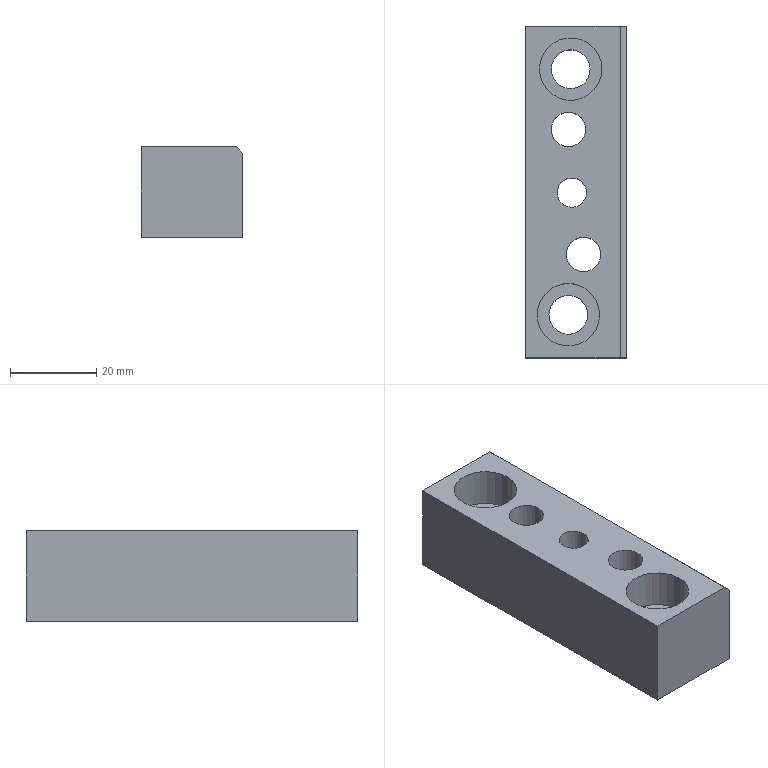Part | NX | features 23 2 | 1 solid | 16 faces | box 23.541 x 77 x 21 mm | volume 30606 mm3 | plane 9 | cylinder 7 | commonest cylinder face diameters 8.001 x2 9 x2 14.5 x2 6.8 x1
STEP:
#1=CARTESIAN_POINT('',(1071.25,287.,-2.5));
#2=VERTEX_POINT('',#1);
#3=CARTESIAN_POINT('',(1064.,287.,-2.5));
#4=DIRECTION('',(0.,0.,1.));
#5=DIRECTION('',(1.,0.,0.));
#6=AXIS2_PLACEMENT_3D('',#3,#4,#5);
#7=CIRCLE('',#6,7.25);
#8=EDGE_CURVE('',#2,#2,#7,.T.);
#9=ORIENTED_EDGE('',*,*,#8,.F.);
#10=EDGE_LOOP('',(#9));
#11=FACE_BOUND('',#10,.T.);
#12=CARTESIAN_POINT('',(1071.542,301.,-2.5));
#13=VERTEX_POINT('',#12);
#14=CARTESIAN_POINT('',(1067.541,301.,-2.5));
#15=DIRECTION('',(0.,0.,-1.));
#16=DIRECTION('',(1.,0.,0.));
#17=AXIS2_PLACEMENT_3D('',#14,#15,#16);
#18=CIRCLE('',#17,4.);
#19=EDGE_CURVE('',#13,#13,#18,.T.);
#20=ORIENTED_EDGE('',*,*,#19,.T.);
#21=EDGE_LOOP('',(#20));
#22=FACE_BOUND('',#21,.T.);
#23=CARTESIAN_POINT('',(1076.041,277.,-2.5));
#24=VERTEX_POINT('',#23);
#25=CARTESIAN_POINT('',(1076.041,354.,-2.5));
#26=VERTEX_POINT('',#25);
#27=CARTESIAN_POINT('',(1076.041,-425.,-2.5));
#28=DIRECTION('',(0.,1.,0.));
#29=VECTOR('',#28,1000.);
#30=LINE('',#27,#29);
#31=EDGE_CURVE('',#24,#26,#30,.T.);
#32=ORIENTED_EDGE('',*,*,#31,.T.);
#33=CARTESIAN_POINT('',(1054.,354.,-2.5));
#34=VERTEX_POINT('',#33);
#35=CARTESIAN_POINT('',(1166.5,354.,-2.5));
#36=DIRECTION('',(1.,0.,0.));
#37=VECTOR('',#36,1000.);
#38=LINE('',#35,#37);
#39=EDGE_CURVE('',#34,#26,#38,.T.);
#40=ORIENTED_EDGE('',*,*,#39,.F.);
#41=CARTESIAN_POINT('',(1054.,277.,-2.5));
#42=VERTEX_POINT('',#41);
#43=CARTESIAN_POINT('',(1054.,328.5,-2.5));
#44=DIRECTION('',(0.,-1.,0.));
#45=VECTOR('',#44,1000.);
#46=LINE('',#43,#45);
#47=EDGE_CURVE('',#34,#42,#46,.T.);
#48=ORIENTED_EDGE('',*,*,#47,.T.);
#49=CARTESIAN_POINT('',(1166.5,277.,-2.5));
#50=DIRECTION('',(1.,0.,0.));
#51=VECTOR('',#50,1000.);
#52=LINE('',#49,#51);
#53=EDGE_CURVE('',#42,#24,#52,.T.);
#54=ORIENTED_EDGE('',*,*,#53,.T.);
#55=EDGE_LOOP('',(#32,#40,#48,#54));
#56=FACE_BOUND('',#55,.T.);
#57=CARTESIAN_POINT('',(1071.791,344.,-2.5));
#58=VERTEX_POINT('',#57);
#59=CARTESIAN_POINT('',(1064.541,344.,-2.5));
#60=DIRECTION('',(0.,0.,1.));
#61=DIRECTION('',(1.,0.,0.));
#62=AXIS2_PLACEMENT_3D('',#59,#60,#61);
#63=CIRCLE('',#62,7.25);
#64=EDGE_CURVE('',#58,#58,#63,.T.);
#65=ORIENTED_EDGE('',*,*,#64,.F.);
#66=EDGE_LOOP('',(#65));
#67=FACE_BOUND('',#66,.T.);
#68=CARTESIAN_POINT('',(1068.001,330.,-2.5));
#69=VERTEX_POINT('',#68);
#70=CARTESIAN_POINT('',(1064.,330.,-2.5));
#71=DIRECTION('',(0.,0.,-1.));
#72=DIRECTION('',(1.,0.,0.));
#73=AXIS2_PLACEMENT_3D('',#70,#71,#72);
#74=CIRCLE('',#73,4.);
#75=EDGE_CURVE('',#69,#69,#74,.T.);
#76=ORIENTED_EDGE('',*,*,#75,.T.);
#77=EDGE_LOOP('',(#76));
#78=FACE_BOUND('',#77,.T.);
#79=CARTESIAN_POINT('',(1068.223,315.331,-2.5));
#80=VERTEX_POINT('',#79);
#81=CARTESIAN_POINT('',(1064.823,315.331,-2.5));
#82=DIRECTION('',(0.,0.,1.));
#83=DIRECTION('',(1.,0.,0.));
#84=AXIS2_PLACEMENT_3D('',#81,#82,#83);
#85=CIRCLE('',#84,3.4);
#86=EDGE_CURVE('',#80,#80,#85,.T.);
#87=ORIENTED_EDGE('',*,*,#86,.F.);
#88=EDGE_LOOP('',(#87));
#89=FACE_BOUND('',#88,.T.);
#90=CARTESIAN_POINT('',(1166.5,279.5,-2.5));
#91=DIRECTION('',(0.,0.,1.));
#92=DIRECTION('',(-1.,0.,0.));
#93=AXIS2_PLACEMENT_3D('',#90,#91,#92);
#94=PLANE('',#93);
#95=ADVANCED_FACE('',(#11,#22,#56,#67,#78,#89),#94,.T.);
#96=CARTESIAN_POINT('',(1054.,354.,-23.5));
#97=VERTEX_POINT('',#96);
#98=CARTESIAN_POINT('',(1054.,354.,-33.5));
#99=DIRECTION('',(0.,0.,-1.));
#100=VECTOR('',#99,1000.);
#101=LINE('',#98,#100);
#102=EDGE_CURVE('',#34,#97,#101,.T.);
#103=ORIENTED_EDGE('',*,*,#102,.F.);
#104=ORIENTED_EDGE('',*,*,#39,.T.);
#105=CARTESIAN_POINT('',(1077.541,354.,-4.));
#106=VERTEX_POINT('',#105);
#107=CARTESIAN_POINT('',(1077.041,354.,-3.5));
#108=DIRECTION('',(0.7071,0.,-0.7071));
#109=VECTOR('',#108,1000.);
#110=LINE('',#107,#109);
#111=EDGE_CURVE('',#26,#106,#110,.T.);
#112=ORIENTED_EDGE('',*,*,#111,.T.);
#113=CARTESIAN_POINT('',(1077.541,354.,-23.5));
#114=VERTEX_POINT('',#113);
#115=CARTESIAN_POINT('',(1077.541,354.,-43.));
#116=DIRECTION('',(0.,0.,1.));
#117=VECTOR('',#116,1000.);
#118=LINE('',#115,#117);
#119=EDGE_CURVE('',#114,#106,#118,.T.);
#120=ORIENTED_EDGE('',*,*,#119,.F.);
#121=CARTESIAN_POINT('',(1136.,354.,-23.5));
#122=DIRECTION('',(-1.,0.,0.));
#123=VECTOR('',#122,1000.);
#124=LINE('',#121,#123);
#125=EDGE_CURVE('',#114,#97,#124,.T.);
#126=ORIENTED_EDGE('',*,*,#125,.T.);
#127=EDGE_LOOP('',(#103,#104,#112,#120,#126));
#128=FACE_BOUND('',#127,.T.);
#129=CARTESIAN_POINT('',(1033.,354.,0.));
#130=DIRECTION('',(0.,1.,0.));
#131=DIRECTION('',(0.,0.,-1.));
#132=AXIS2_PLACEMENT_3D('',#129,#130,#131);
#133=PLANE('',#132);
#134=ADVANCED_FACE('',(#128),#133,.T.);
#135=CARTESIAN_POINT('',(1054.,277.,-23.5));
#136=VERTEX_POINT('',#135);
#137=CARTESIAN_POINT('',(1054.,277.,-33.5));
#138=DIRECTION('',(0.,0.,-1.));
#139=VECTOR('',#138,1000.);
#140=LINE('',#137,#139);
#141=EDGE_CURVE('',#42,#136,#140,.T.);
#142=ORIENTED_EDGE('',*,*,#141,.T.);
#143=CARTESIAN_POINT('',(1077.541,277.,-23.5));
#144=VERTEX_POINT('',#143);
#145=CARTESIAN_POINT('',(1136.,277.,-23.5));
#146=DIRECTION('',(-1.,0.,0.));
#147=VECTOR('',#146,1000.);
#148=LINE('',#145,#147);
#149=EDGE_CURVE('',#144,#136,#148,.T.);
#150=ORIENTED_EDGE('',*,*,#149,.F.);
#151=CARTESIAN_POINT('',(1077.541,277.,-4.));
#152=VERTEX_POINT('',#151);
#153=CARTESIAN_POINT('',(1077.541,277.,-43.));
#154=DIRECTION('',(0.,0.,-1.));
#155=VECTOR('',#154,1000.);
#156=LINE('',#153,#155);
#157=EDGE_CURVE('',#152,#144,#156,.T.);
#158=ORIENTED_EDGE('',*,*,#157,.F.);
#159=CARTESIAN_POINT('',(1077.041,277.,-3.5));
#160=DIRECTION('',(-0.7071,0.,0.7071));
#161=VECTOR('',#160,1000.);
#162=LINE('',#159,#161);
#163=EDGE_CURVE('',#152,#24,#162,.T.);
#164=ORIENTED_EDGE('',*,*,#163,.T.);
#165=ORIENTED_EDGE('',*,*,#53,.F.);
#166=EDGE_LOOP('',(#142,#150,#158,#164,#165));
#167=FACE_BOUND('',#166,.T.);
#168=CARTESIAN_POINT('',(1027.,277.,0.));
#169=DIRECTION('',(0.,1.,0.));
#170=DIRECTION('',(0.,0.,-1.));
#171=AXIS2_PLACEMENT_3D('',#168,#169,#170);
#172=PLANE('',#171);
#173=ADVANCED_FACE('',(#167),#172,.F.);
#174=CARTESIAN_POINT('',(1077.541,328.5,-23.5));
#175=DIRECTION('',(0.,-1.,0.));
#176=VECTOR('',#175,1000.);
#177=LINE('',#174,#176);
#178=EDGE_CURVE('',#114,#144,#177,.T.);
#179=ORIENTED_EDGE('',*,*,#178,.F.);
#180=ORIENTED_EDGE('',*,*,#119,.T.);
#181=CARTESIAN_POINT('',(1077.541,-425.,-4.));
#182=DIRECTION('',(0.,-1.,0.));
#183=VECTOR('',#182,1000.);
#184=LINE('',#181,#183);
#185=EDGE_CURVE('',#106,#152,#184,.T.);
#186=ORIENTED_EDGE('',*,*,#185,.T.);
#187=ORIENTED_EDGE('',*,*,#157,.T.);
#188=EDGE_LOOP('',(#179,#180,#186,#187));
#189=FACE_BOUND('',#188,.T.);
#190=CARTESIAN_POINT('',(1077.541,275.983,-43.));
#191=DIRECTION('',(1.,0.,0.));
#192=DIRECTION('',(0.,0.,1.));
#193=AXIS2_PLACEMENT_3D('',#190,#191,#192);
#194=PLANE('',#193);
#195=ADVANCED_FACE('',(#189),#194,.T.);
#196=ORIENTED_EDGE('',*,*,#185,.F.);
#197=ORIENTED_EDGE('',*,*,#111,.F.);
#198=ORIENTED_EDGE('',*,*,#31,.F.);
#199=ORIENTED_EDGE('',*,*,#163,.F.);
#200=EDGE_LOOP('',(#196,#197,#198,#199));
#201=FACE_BOUND('',#200,.T.);
#202=CARTESIAN_POINT('',(1077.041,-425.,-3.5));
#203=DIRECTION('',(0.7071,0.,0.7071));
#204=DIRECTION('',(0.,-1.,0.));
#205=AXIS2_PLACEMENT_3D('',#202,#203,#204);
#206=PLANE('',#205);
#207=ADVANCED_FACE('',(#201),#206,.T.);
#208=ORIENTED_EDGE('',*,*,#47,.F.);
#209=ORIENTED_EDGE('',*,*,#102,.T.);
#210=CARTESIAN_POINT('',(1054.,328.5,-23.5));
#211=DIRECTION('',(0.,1.,0.));
#212=VECTOR('',#211,1000.);
#213=LINE('',#210,#212);
#214=EDGE_CURVE('',#136,#97,#213,.T.);
#215=ORIENTED_EDGE('',*,*,#214,.F.);
#216=ORIENTED_EDGE('',*,*,#141,.F.);
#217=EDGE_LOOP('',(#208,#209,#215,#216));
#218=FACE_BOUND('',#217,.T.);
#219=CARTESIAN_POINT('',(1054.,328.5,-33.5));
#220=DIRECTION('',(-1.,0.,0.));
#221=DIRECTION('',(0.,0.,-1.));
#222=AXIS2_PLACEMENT_3D('',#219,#220,#221);
#223=PLANE('',#222);
#224=ADVANCED_FACE('',(#218),#223,.T.);
#225=CARTESIAN_POINT('',(1061.423,315.331,-23.5));
#226=VERTEX_POINT('',#225);
#227=CARTESIAN_POINT('',(1064.823,315.331,-23.5));
#228=DIRECTION('',(0.,0.,1.));
#229=DIRECTION('',(-1.,0.,0.));
#230=AXIS2_PLACEMENT_3D('',#227,#228,#229);
#231=CIRCLE('',#230,3.4);
#232=EDGE_CURVE('',#226,#226,#231,.T.);
#233=ORIENTED_EDGE('',*,*,#232,.T.);
#234=EDGE_LOOP('',(#233));
#235=FACE_BOUND('',#234,.T.);
#236=CARTESIAN_POINT('',(1059.999,330.,-23.5));
#237=VERTEX_POINT('',#236);
#238=CARTESIAN_POINT('',(1064.,330.,-23.5));
#239=DIRECTION('',(0.,0.,1.));
#240=DIRECTION('',(-1.,0.,0.));
#241=AXIS2_PLACEMENT_3D('',#238,#239,#240);
#242=CIRCLE('',#241,4.);
#243=EDGE_CURVE('',#237,#237,#242,.T.);
#244=ORIENTED_EDGE('',*,*,#243,.T.);
#245=EDGE_LOOP('',(#244));
#246=FACE_BOUND('',#245,.T.);
#247=CARTESIAN_POINT('',(1059.5,287.,-23.5));
#248=VERTEX_POINT('',#247);
#249=CARTESIAN_POINT('',(1064.,287.,-23.5));
#250=DIRECTION('',(0.,0.,1.));
#251=DIRECTION('',(-1.,0.,0.));
#252=AXIS2_PLACEMENT_3D('',#249,#250,#251);
#253=CIRCLE('',#252,4.5);
#254=EDGE_CURVE('',#248,#248,#253,.T.);
#255=ORIENTED_EDGE('',*,*,#254,.T.);
#256=EDGE_LOOP('',(#255));
#257=FACE_BOUND('',#256,.T.);
#258=CARTESIAN_POINT('',(1063.541,301.,-23.5));
#259=VERTEX_POINT('',#258);
#260=CARTESIAN_POINT('',(1067.541,301.,-23.5));
#261=DIRECTION('',(0.,0.,1.));
#262=DIRECTION('',(-1.,0.,0.));
#263=AXIS2_PLACEMENT_3D('',#260,#261,#262);
#264=CIRCLE('',#263,4.);
#265=EDGE_CURVE('',#259,#259,#264,.T.);
#266=ORIENTED_EDGE('',*,*,#265,.T.);
#267=EDGE_LOOP('',(#266));
#268=FACE_BOUND('',#267,.T.);
#269=CARTESIAN_POINT('',(1060.041,344.,-23.5));
#270=VERTEX_POINT('',#269);
#271=CARTESIAN_POINT('',(1064.541,344.,-23.5));
#272=DIRECTION('',(0.,0.,1.));
#273=DIRECTION('',(-1.,0.,0.));
#274=AXIS2_PLACEMENT_3D('',#271,#272,#273);
#275=CIRCLE('',#274,4.5);
#276=EDGE_CURVE('',#270,#270,#275,.T.);
#277=ORIENTED_EDGE('',*,*,#276,.T.);
#278=EDGE_LOOP('',(#277));
#279=FACE_BOUND('',#278,.T.);
#280=ORIENTED_EDGE('',*,*,#214,.T.);
#281=ORIENTED_EDGE('',*,*,#125,.F.);
#282=ORIENTED_EDGE('',*,*,#178,.T.);
#283=ORIENTED_EDGE('',*,*,#149,.T.);
#284=EDGE_LOOP('',(#280,#281,#282,#283));
#285=FACE_BOUND('',#284,.T.);
#286=CARTESIAN_POINT('',(1136.,328.5,-23.5));
#287=DIRECTION('',(0.,0.,-1.));
#288=DIRECTION('',(1.,0.,0.));
#289=AXIS2_PLACEMENT_3D('',#286,#287,#288);
#290=PLANE('',#289);
#291=ADVANCED_FACE('',(#235,#246,#257,#268,#279,#285),#290,.T.);
#292=ORIENTED_EDGE('',*,*,#276,.F.);
#293=EDGE_LOOP('',(#292));
#294=FACE_BOUND('',#293,.T.);
#295=CARTESIAN_POINT('',(1060.041,344.,-11.5));
#296=VERTEX_POINT('',#295);
#297=CARTESIAN_POINT('',(1064.541,344.,-11.5));
#298=DIRECTION('',(0.,0.,1.));
#299=DIRECTION('',(-1.,0.,0.));
#300=AXIS2_PLACEMENT_3D('',#297,#298,#299);
#301=CIRCLE('',#300,4.5);
#302=EDGE_CURVE('',#296,#296,#301,.T.);
#303=ORIENTED_EDGE('',*,*,#302,.T.);
#304=EDGE_LOOP('',(#303));
#305=FACE_BOUND('',#304,.T.);
#306=CARTESIAN_POINT('',(1064.541,344.,-0.5));
#307=DIRECTION('',(0.,0.,-1.));
#308=DIRECTION('',(-1.,0.,0.));
#309=AXIS2_PLACEMENT_3D('',#306,#307,#308);
#310=CYLINDRICAL_SURFACE('',#309,4.5);
#311=ADVANCED_FACE('',(#294,#305),#310,.F.);
#312=ORIENTED_EDGE('',*,*,#302,.F.);
#313=EDGE_LOOP('',(#312));
#314=FACE_BOUND('',#313,.T.);
#315=CARTESIAN_POINT('',(1057.291,344.,-11.5));
#316=VERTEX_POINT('',#315);
#317=CARTESIAN_POINT('',(1064.541,344.,-11.5));
#318=DIRECTION('',(0.,0.,1.));
#319=DIRECTION('',(-1.,0.,0.));
#320=AXIS2_PLACEMENT_3D('',#317,#318,#319);
#321=CIRCLE('',#320,7.25);
#322=EDGE_CURVE('',#316,#316,#321,.T.);
#323=ORIENTED_EDGE('',*,*,#322,.T.);
#324=EDGE_LOOP('',(#323));
#325=FACE_BOUND('',#324,.T.);
#326=CARTESIAN_POINT('',(1064.541,344.,-11.5));
#327=DIRECTION('',(0.,0.,-1.));
#328=DIRECTION('',(1.,0.,0.));
#329=AXIS2_PLACEMENT_3D('',#326,#327,#328);
#330=PLANE('',#329);
#331=ADVANCED_FACE('',(#314,#325),#330,.F.);
#332=ORIENTED_EDGE('',*,*,#322,.F.);
#333=EDGE_LOOP('',(#332));
#334=FACE_BOUND('',#333,.T.);
#335=ORIENTED_EDGE('',*,*,#64,.T.);
#336=EDGE_LOOP('',(#335));
#337=FACE_BOUND('',#336,.T.);
#338=CARTESIAN_POINT('',(1064.541,344.,-2.5));
#339=DIRECTION('',(0.,0.,-1.));
#340=DIRECTION('',(-1.,0.,0.));
#341=AXIS2_PLACEMENT_3D('',#338,#339,#340);
#342=CYLINDRICAL_SURFACE('',#341,7.25);
#343=ADVANCED_FACE('',(#334,#337),#342,.F.);
#344=ORIENTED_EDGE('',*,*,#19,.F.);
#345=EDGE_LOOP('',(#344));
#346=FACE_BOUND('',#345,.T.);
#347=ORIENTED_EDGE('',*,*,#265,.F.);
#348=EDGE_LOOP('',(#347));
#349=FACE_BOUND('',#348,.T.);
#350=CARTESIAN_POINT('',(1067.541,301.,-0.5));
#351=DIRECTION('',(0.,0.,-1.));
#352=DIRECTION('',(-1.,0.,0.));
#353=AXIS2_PLACEMENT_3D('',#350,#351,#352);
#354=CYLINDRICAL_SURFACE('',#353,4.);
#355=ADVANCED_FACE('',(#346,#349),#354,.F.);
#356=ORIENTED_EDGE('',*,*,#254,.F.);
#357=EDGE_LOOP('',(#356));
#358=FACE_BOUND('',#357,.T.);
#359=CARTESIAN_POINT('',(1059.5,287.,-11.5));
#360=VERTEX_POINT('',#359);
#361=CARTESIAN_POINT('',(1064.,287.,-11.5));
#362=DIRECTION('',(0.,0.,1.));
#363=DIRECTION('',(-1.,0.,0.));
#364=AXIS2_PLACEMENT_3D('',#361,#362,#363);
#365=CIRCLE('',#364,4.5);
#366=EDGE_CURVE('',#360,#360,#365,.T.);
#367=ORIENTED_EDGE('',*,*,#366,.T.);
#368=EDGE_LOOP('',(#367));
#369=FACE_BOUND('',#368,.T.);
#370=CARTESIAN_POINT('',(1064.,287.,-0.5));
#371=DIRECTION('',(0.,0.,-1.));
#372=DIRECTION('',(-1.,0.,0.));
#373=AXIS2_PLACEMENT_3D('',#370,#371,#372);
#374=CYLINDRICAL_SURFACE('',#373,4.5);
#375=ADVANCED_FACE('',(#358,#369),#374,.F.);
#376=ORIENTED_EDGE('',*,*,#366,.F.);
#377=EDGE_LOOP('',(#376));
#378=FACE_BOUND('',#377,.T.);
#379=CARTESIAN_POINT('',(1056.75,287.,-11.5));
#380=VERTEX_POINT('',#379);
#381=CARTESIAN_POINT('',(1064.,287.,-11.5));
#382=DIRECTION('',(0.,0.,1.));
#383=DIRECTION('',(-1.,0.,0.));
#384=AXIS2_PLACEMENT_3D('',#381,#382,#383);
#385=CIRCLE('',#384,7.25);
#386=EDGE_CURVE('',#380,#380,#385,.T.);
#387=ORIENTED_EDGE('',*,*,#386,.T.);
#388=EDGE_LOOP('',(#387));
#389=FACE_BOUND('',#388,.T.);
#390=CARTESIAN_POINT('',(1064.,287.,-11.5));
#391=DIRECTION('',(0.,0.,-1.));
#392=DIRECTION('',(1.,0.,0.));
#393=AXIS2_PLACEMENT_3D('',#390,#391,#392);
#394=PLANE('',#393);
#395=ADVANCED_FACE('',(#378,#389),#394,.F.);
#396=ORIENTED_EDGE('',*,*,#386,.F.);
#397=EDGE_LOOP('',(#396));
#398=FACE_BOUND('',#397,.T.);
#399=ORIENTED_EDGE('',*,*,#8,.T.);
#400=EDGE_LOOP('',(#399));
#401=FACE_BOUND('',#400,.T.);
#402=CARTESIAN_POINT('',(1064.,287.,-2.5));
#403=DIRECTION('',(0.,0.,-1.));
#404=DIRECTION('',(-1.,0.,0.));
#405=AXIS2_PLACEMENT_3D('',#402,#403,#404);
#406=CYLINDRICAL_SURFACE('',#405,7.25);
#407=ADVANCED_FACE('',(#398,#401),#406,.F.);
#408=ORIENTED_EDGE('',*,*,#75,.F.);
#409=EDGE_LOOP('',(#408));
#410=FACE_BOUND('',#409,.T.);
#411=ORIENTED_EDGE('',*,*,#243,.F.);
#412=EDGE_LOOP('',(#411));
#413=FACE_BOUND('',#412,.T.);
#414=CARTESIAN_POINT('',(1064.,330.,-0.5));
#415=DIRECTION('',(0.,0.,-1.));
#416=DIRECTION('',(-1.,0.,0.));
#417=AXIS2_PLACEMENT_3D('',#414,#415,#416);
#418=CYLINDRICAL_SURFACE('',#417,4.);
#419=ADVANCED_FACE('',(#410,#413),#418,.F.);
#420=ORIENTED_EDGE('',*,*,#232,.F.);
#421=EDGE_LOOP('',(#420));
#422=FACE_BOUND('',#421,.T.);
#423=ORIENTED_EDGE('',*,*,#86,.T.);
#424=EDGE_LOOP('',(#423));
#425=FACE_BOUND('',#424,.T.);
#426=CARTESIAN_POINT('',(1064.823,315.331,-2.5));
#427=DIRECTION('',(0.,0.,-1.));
#428=DIRECTION('',(-1.,0.,0.));
#429=AXIS2_PLACEMENT_3D('',#426,#427,#428);
#430=CYLINDRICAL_SURFACE('',#429,3.4);
#431=ADVANCED_FACE('',(#422,#425),#430,.F.);
#432=CLOSED_SHELL('',(#95,#134,#173,#195,#207,#224,#291,#311,#331,#343,#355,#375,#395,#407,#419,#431));
#433=MANIFOLD_SOLID_BREP('',#432);
#434=(LENGTH_UNIT()NAMED_UNIT(*)SI_UNIT(.MILLI.,.METRE.));
#435=UNCERTAINTY_MEASURE_WITH_UNIT(LENGTH_MEASURE(0.00001),#434,'','');
#436=(NAMED_UNIT(*)PLANE_ANGLE_UNIT()SI_UNIT($,.RADIAN.));
#437=(NAMED_UNIT(*)SI_UNIT($,.STERADIAN.)SOLID_ANGLE_UNIT());
#438=(GEOMETRIC_REPRESENTATION_CONTEXT(3)GLOBAL_UNCERTAINTY_ASSIGNED_CONTEXT((#435))GLOBAL_UNIT_ASSIGNED_CONTEXT((#434,#436,#437))REPRESENTATION_CONTEXT('',''));
#439=ADVANCED_BREP_SHAPE_REPRESENTATION('',(#433),#438);